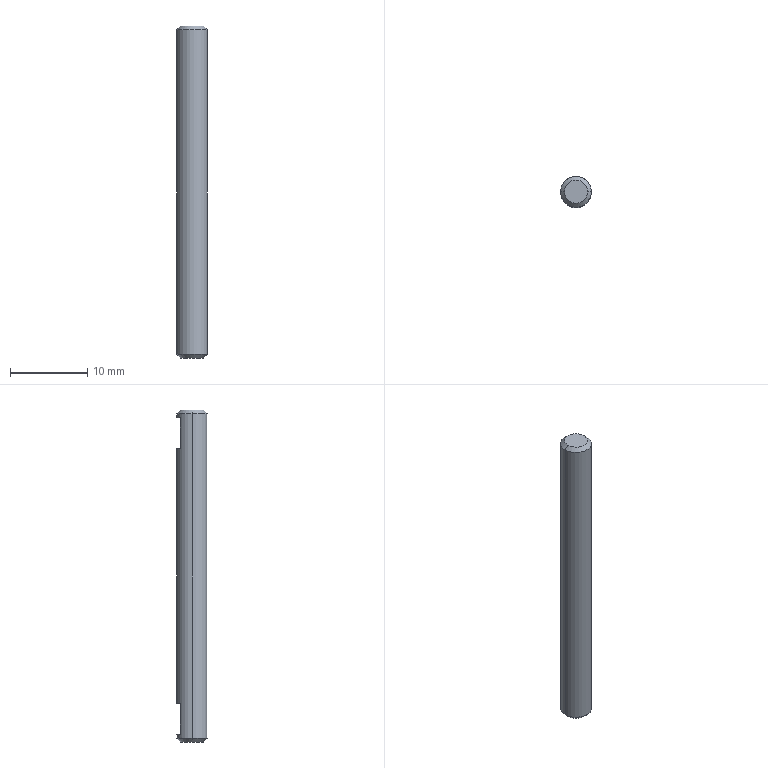Part | SolidWorks | features Chamfer 1, Extrusion 1, ICE 1 | 1 solid | 14 faces | box 4 x 4 x 43 mm | volume 530.221 mm3 | plane 8 | cone 4 | cylinder 2 | commonest cylinder face diameters 4 x2
STEP:
#1=CARTESIAN_POINT('',(-1.5,0.,-21.5));
#2=VERTEX_POINT('',#1);
#3=CARTESIAN_POINT('',(1.5,0.,-21.5));
#4=VERTEX_POINT('',#3);
#5=CARTESIAN_POINT('',(0.,0.,-21.5));
#6=DIRECTION('',(0.,0.,-1.));
#7=DIRECTION('',(1.,0.,0.));
#8=AXIS2_PLACEMENT_3D('',#5,#6,#7);
#9=CIRCLE('',#8,1.5);
#10=EDGE_CURVE('',#2,#4,#9,.T.);
#11=ORIENTED_EDGE('',*,*,#10,.F.);
#12=CARTESIAN_POINT('',(-2.,0.,-21.));
#13=VERTEX_POINT('',#12);
#14=CARTESIAN_POINT('',(-2.,0.,-21.));
#15=DIRECTION('',(-0.7071,0.,0.7071));
#16=VECTOR('',#15,1000.);
#17=LINE('',#14,#16);
#18=EDGE_CURVE('',#2,#13,#17,.T.);
#19=ORIENTED_EDGE('',*,*,#18,.T.);
#20=CARTESIAN_POINT('',(2.,0.,-21.));
#21=VERTEX_POINT('',#20);
#22=CARTESIAN_POINT('',(0.,0.,-21.));
#23=DIRECTION('',(0.,0.,1.));
#24=DIRECTION('',(1.,0.,0.));
#25=AXIS2_PLACEMENT_3D('',#22,#23,#24);
#26=CIRCLE('',#25,2.);
#27=EDGE_CURVE('',#21,#13,#26,.T.);
#28=ORIENTED_EDGE('',*,*,#27,.F.);
#29=CARTESIAN_POINT('',(2.,0.,-21.));
#30=DIRECTION('',(0.7071,0.,0.7071));
#31=VECTOR('',#30,1000.);
#32=LINE('',#29,#31);
#33=EDGE_CURVE('',#4,#21,#32,.T.);
#34=ORIENTED_EDGE('',*,*,#33,.F.);
#35=EDGE_LOOP('',(#11,#19,#28,#34));
#36=FACE_OUTER_BOUND('',#35,.T.);
#37=CARTESIAN_POINT('',(0.,0.,-21.));
#38=DIRECTION('',(0.,0.,1.));
#39=DIRECTION('',(1.,0.,0.));
#40=AXIS2_PLACEMENT_3D('',#37,#38,#39);
#41=CONICAL_SURFACE('',#40,2.,0.7854);
#42=ADVANCED_FACE('',(#36),#41,.T.);
#43=CARTESIAN_POINT('',(1.5,0.,21.5));
#44=VERTEX_POINT('',#43);
#45=CARTESIAN_POINT('',(-1.5,0.,21.5));
#46=VERTEX_POINT('',#45);
#47=CARTESIAN_POINT('',(0.,0.,21.5));
#48=DIRECTION('',(0.,0.,1.));
#49=DIRECTION('',(1.,0.,0.));
#50=AXIS2_PLACEMENT_3D('',#47,#48,#49);
#51=CIRCLE('',#50,1.5);
#52=EDGE_CURVE('',#44,#46,#51,.T.);
#53=ORIENTED_EDGE('',*,*,#52,.F.);
#54=CARTESIAN_POINT('',(2.,0.,21.));
#55=VERTEX_POINT('',#54);
#56=CARTESIAN_POINT('',(1.5,0.,21.5));
#57=DIRECTION('',(0.7071,0.,-0.7071));
#58=VECTOR('',#57,1000.);
#59=LINE('',#56,#58);
#60=EDGE_CURVE('',#44,#55,#59,.T.);
#61=ORIENTED_EDGE('',*,*,#60,.T.);
#62=CARTESIAN_POINT('',(-2.,0.,21.));
#63=VERTEX_POINT('',#62);
#64=CARTESIAN_POINT('',(0.,0.,21.));
#65=DIRECTION('',(0.,0.,-1.));
#66=DIRECTION('',(1.,0.,0.));
#67=AXIS2_PLACEMENT_3D('',#64,#65,#66);
#68=CIRCLE('',#67,2.);
#69=EDGE_CURVE('',#63,#55,#68,.T.);
#70=ORIENTED_EDGE('',*,*,#69,.F.);
#71=CARTESIAN_POINT('',(-1.5,0.,21.5));
#72=DIRECTION('',(-0.7071,0.,-0.7071));
#73=VECTOR('',#72,1000.);
#74=LINE('',#71,#73);
#75=EDGE_CURVE('',#46,#63,#74,.T.);
#76=ORIENTED_EDGE('',*,*,#75,.F.);
#77=EDGE_LOOP('',(#53,#61,#70,#76));
#78=FACE_OUTER_BOUND('',#77,.T.);
#79=CARTESIAN_POINT('',(0.,0.,21.5));
#80=DIRECTION('',(0.,0.,-1.));
#81=DIRECTION('',(-1.,0.,0.));
#82=AXIS2_PLACEMENT_3D('',#79,#80,#81);
#83=CONICAL_SURFACE('',#82,1.5,0.7854);
#84=ADVANCED_FACE('',(#78),#83,.T.);
#85=CARTESIAN_POINT('',(1.323,1.5,-16.5));
#86=VERTEX_POINT('',#85);
#87=CARTESIAN_POINT('',(1.323,1.5,-20.5));
#88=VERTEX_POINT('',#87);
#89=CARTESIAN_POINT('',(1.323,1.5,21.5));
#90=DIRECTION('',(0.,0.,-1.));
#91=VECTOR('',#90,1000.);
#92=LINE('',#89,#91);
#93=EDGE_CURVE('',#86,#88,#92,.T.);
#94=ORIENTED_EDGE('',*,*,#93,.F.);
#95=CARTESIAN_POINT('',(-1.323,1.5,-16.5));
#96=VERTEX_POINT('',#95);
#97=CARTESIAN_POINT('',(0.,0.,-16.5));
#98=DIRECTION('',(0.,0.,1.));
#99=DIRECTION('',(1.,0.,0.));
#100=AXIS2_PLACEMENT_3D('',#97,#98,#99);
#101=CIRCLE('',#100,2.);
#102=EDGE_CURVE('',#86,#96,#101,.T.);
#103=ORIENTED_EDGE('',*,*,#102,.T.);
#104=CARTESIAN_POINT('',(-1.323,1.5,-20.5));
#105=VERTEX_POINT('',#104);
#106=CARTESIAN_POINT('',(-1.323,1.5,21.5));
#107=DIRECTION('',(0.,0.,1.));
#108=VECTOR('',#107,1000.);
#109=LINE('',#106,#108);
#110=EDGE_CURVE('',#105,#96,#109,.T.);
#111=ORIENTED_EDGE('',*,*,#110,.F.);
#112=CARTESIAN_POINT('',(0.,0.,-20.5));
#113=DIRECTION('',(0.,0.,-1.));
#114=DIRECTION('',(-1.,0.,0.));
#115=AXIS2_PLACEMENT_3D('',#112,#113,#114);
#116=CIRCLE('',#115,2.);
#117=EDGE_CURVE('',#105,#88,#116,.T.);
#118=ORIENTED_EDGE('',*,*,#117,.T.);
#119=EDGE_LOOP('',(#94,#103,#111,#118));
#120=FACE_BOUND('',#119,.T.);
#121=CARTESIAN_POINT('',(1.323,1.5,20.5));
#122=VERTEX_POINT('',#121);
#123=CARTESIAN_POINT('',(1.323,1.5,16.5));
#124=VERTEX_POINT('',#123);
#125=CARTESIAN_POINT('',(1.323,1.5,21.5));
#126=DIRECTION('',(0.,0.,-1.));
#127=VECTOR('',#126,1000.);
#128=LINE('',#125,#127);
#129=EDGE_CURVE('',#122,#124,#128,.T.);
#130=ORIENTED_EDGE('',*,*,#129,.F.);
#131=CARTESIAN_POINT('',(-1.323,1.5,20.5));
#132=VERTEX_POINT('',#131);
#133=CARTESIAN_POINT('',(0.,0.,20.5));
#134=DIRECTION('',(0.,0.,1.));
#135=DIRECTION('',(1.,0.,0.));
#136=AXIS2_PLACEMENT_3D('',#133,#134,#135);
#137=CIRCLE('',#136,2.);
#138=EDGE_CURVE('',#122,#132,#137,.T.);
#139=ORIENTED_EDGE('',*,*,#138,.T.);
#140=CARTESIAN_POINT('',(-1.323,1.5,16.5));
#141=VERTEX_POINT('',#140);
#142=CARTESIAN_POINT('',(-1.323,1.5,21.5));
#143=DIRECTION('',(0.,0.,1.));
#144=VECTOR('',#143,1000.);
#145=LINE('',#142,#144);
#146=EDGE_CURVE('',#141,#132,#145,.T.);
#147=ORIENTED_EDGE('',*,*,#146,.F.);
#148=CARTESIAN_POINT('',(0.,0.,16.5));
#149=DIRECTION('',(0.,0.,-1.));
#150=DIRECTION('',(-1.,0.,0.));
#151=AXIS2_PLACEMENT_3D('',#148,#149,#150);
#152=CIRCLE('',#151,2.);
#153=EDGE_CURVE('',#141,#124,#152,.T.);
#154=ORIENTED_EDGE('',*,*,#153,.T.);
#155=EDGE_LOOP('',(#130,#139,#147,#154));
#156=FACE_BOUND('',#155,.T.);
#157=ORIENTED_EDGE('',*,*,#69,.T.);
#158=CARTESIAN_POINT('',(2.,0.,21.5));
#159=DIRECTION('',(0.,0.,-1.));
#160=VECTOR('',#159,1000.);
#161=LINE('',#158,#160);
#162=EDGE_CURVE('',#55,#21,#161,.T.);
#163=ORIENTED_EDGE('',*,*,#162,.T.);
#164=ORIENTED_EDGE('',*,*,#27,.T.);
#165=CARTESIAN_POINT('',(-2.,0.,21.5));
#166=DIRECTION('',(0.,0.,-1.));
#167=VECTOR('',#166,1000.);
#168=LINE('',#165,#167);
#169=EDGE_CURVE('',#63,#13,#168,.T.);
#170=ORIENTED_EDGE('',*,*,#169,.F.);
#171=EDGE_LOOP('',(#157,#163,#164,#170));
#172=FACE_OUTER_BOUND('',#171,.T.);
#173=CARTESIAN_POINT('',(0.,0.,21.5));
#174=DIRECTION('',(0.,0.,-1.));
#175=DIRECTION('',(-1.,0.,0.));
#176=AXIS2_PLACEMENT_3D('',#173,#174,#175);
#177=CYLINDRICAL_SURFACE('',#176,2.);
#178=ADVANCED_FACE('',(#120,#156,#172),#177,.T.);
#179=ORIENTED_EDGE('',*,*,#162,.F.);
#180=CARTESIAN_POINT('',(0.,0.,21.));
#181=DIRECTION('',(0.,0.,-1.));
#182=DIRECTION('',(1.,0.,0.));
#183=AXIS2_PLACEMENT_3D('',#180,#181,#182);
#184=CIRCLE('',#183,2.);
#185=EDGE_CURVE('',#55,#63,#184,.T.);
#186=ORIENTED_EDGE('',*,*,#185,.T.);
#187=ORIENTED_EDGE('',*,*,#169,.T.);
#188=CARTESIAN_POINT('',(0.,0.,-21.));
#189=DIRECTION('',(0.,0.,1.));
#190=DIRECTION('',(1.,0.,0.));
#191=AXIS2_PLACEMENT_3D('',#188,#189,#190);
#192=CIRCLE('',#191,2.);
#193=EDGE_CURVE('',#13,#21,#192,.T.);
#194=ORIENTED_EDGE('',*,*,#193,.T.);
#195=EDGE_LOOP('',(#179,#186,#187,#194));
#196=FACE_OUTER_BOUND('',#195,.T.);
#197=CARTESIAN_POINT('',(0.,0.,21.5));
#198=DIRECTION('',(0.,0.,-1.));
#199=DIRECTION('',(-1.,0.,0.));
#200=AXIS2_PLACEMENT_3D('',#197,#198,#199);
#201=CYLINDRICAL_SURFACE('',#200,2.);
#202=ADVANCED_FACE('',(#196),#201,.T.);
#203=CARTESIAN_POINT('',(0.,0.,21.5));
#204=DIRECTION('',(0.,0.,1.));
#205=DIRECTION('',(1.,0.,0.));
#206=AXIS2_PLACEMENT_3D('',#203,#204,#205);
#207=CIRCLE('',#206,1.5);
#208=EDGE_CURVE('',#46,#44,#207,.T.);
#209=ORIENTED_EDGE('',*,*,#208,.T.);
#210=ORIENTED_EDGE('',*,*,#52,.T.);
#211=EDGE_LOOP('',(#209,#210));
#212=FACE_OUTER_BOUND('',#211,.T.);
#213=CARTESIAN_POINT('',(0.,0.,21.5));
#214=DIRECTION('',(0.,0.,1.));
#215=DIRECTION('',(1.,0.,0.));
#216=AXIS2_PLACEMENT_3D('',#213,#214,#215);
#217=PLANE('',#216);
#218=ADVANCED_FACE('',(#212),#217,.T.);
#219=CARTESIAN_POINT('',(0.,0.,-21.5));
#220=DIRECTION('',(0.,0.,-1.));
#221=DIRECTION('',(1.,0.,0.));
#222=AXIS2_PLACEMENT_3D('',#219,#220,#221);
#223=CIRCLE('',#222,1.5);
#224=EDGE_CURVE('',#4,#2,#223,.T.);
#225=ORIENTED_EDGE('',*,*,#224,.T.);
#226=ORIENTED_EDGE('',*,*,#10,.T.);
#227=EDGE_LOOP('',(#225,#226));
#228=FACE_OUTER_BOUND('',#227,.T.);
#229=CARTESIAN_POINT('',(0.,0.,-21.5));
#230=DIRECTION('',(0.,0.,1.));
#231=DIRECTION('',(1.,0.,0.));
#232=AXIS2_PLACEMENT_3D('',#229,#230,#231);
#233=PLANE('',#232);
#234=ADVANCED_FACE('',(#228),#233,.F.);
#235=CARTESIAN_POINT('',(7.709,1.5,20.5));
#236=DIRECTION('',(1.,0.,0.));
#237=VECTOR('',#236,1000.);
#238=LINE('',#235,#237);
#239=EDGE_CURVE('',#132,#122,#238,.T.);
#240=ORIENTED_EDGE('',*,*,#239,.F.);
#241=ORIENTED_EDGE('',*,*,#138,.F.);
#242=EDGE_LOOP('',(#240,#241));
#243=FACE_OUTER_BOUND('',#242,.T.);
#244=CARTESIAN_POINT('',(7.709,1.5,20.5));
#245=DIRECTION('',(0.,0.,1.));
#246=DIRECTION('',(1.,0.,0.));
#247=AXIS2_PLACEMENT_3D('',#244,#245,#246);
#248=PLANE('',#247);
#249=ADVANCED_FACE('',(#243),#248,.F.);
#250=CARTESIAN_POINT('',(7.709,1.5,16.5));
#251=DIRECTION('',(-1.,0.,0.));
#252=VECTOR('',#251,1000.);
#253=LINE('',#250,#252);
#254=EDGE_CURVE('',#124,#141,#253,.T.);
#255=ORIENTED_EDGE('',*,*,#254,.F.);
#256=ORIENTED_EDGE('',*,*,#153,.F.);
#257=EDGE_LOOP('',(#255,#256));
#258=FACE_OUTER_BOUND('',#257,.T.);
#259=CARTESIAN_POINT('',(7.709,1.5,16.5));
#260=DIRECTION('',(0.,0.,-1.));
#261=DIRECTION('',(-1.,0.,0.));
#262=AXIS2_PLACEMENT_3D('',#259,#260,#261);
#263=PLANE('',#262);
#264=ADVANCED_FACE('',(#258),#263,.F.);
#265=ORIENTED_EDGE('',*,*,#129,.T.);
#266=ORIENTED_EDGE('',*,*,#254,.T.);
#267=ORIENTED_EDGE('',*,*,#146,.T.);
#268=ORIENTED_EDGE('',*,*,#239,.T.);
#269=EDGE_LOOP('',(#265,#266,#267,#268));
#270=FACE_OUTER_BOUND('',#269,.T.);
#271=CARTESIAN_POINT('',(7.709,1.5,16.5));
#272=DIRECTION('',(0.,1.,0.));
#273=DIRECTION('',(0.,0.,1.));
#274=AXIS2_PLACEMENT_3D('',#271,#272,#273);
#275=PLANE('',#274);
#276=ADVANCED_FACE('',(#270),#275,.T.);
#277=CARTESIAN_POINT('',(5.032,1.5,-16.5));
#278=DIRECTION('',(1.,0.,0.));
#279=VECTOR('',#278,1000.);
#280=LINE('',#277,#279);
#281=EDGE_CURVE('',#96,#86,#280,.T.);
#282=ORIENTED_EDGE('',*,*,#281,.F.);
#283=ORIENTED_EDGE('',*,*,#102,.F.);
#284=EDGE_LOOP('',(#282,#283));
#285=FACE_OUTER_BOUND('',#284,.T.);
#286=CARTESIAN_POINT('',(5.032,1.5,-16.5));
#287=DIRECTION('',(0.,0.,1.));
#288=DIRECTION('',(1.,0.,0.));
#289=AXIS2_PLACEMENT_3D('',#286,#287,#288);
#290=PLANE('',#289);
#291=ADVANCED_FACE('',(#285),#290,.F.);
#292=CARTESIAN_POINT('',(5.032,1.5,-20.5));
#293=DIRECTION('',(-1.,0.,0.));
#294=VECTOR('',#293,1000.);
#295=LINE('',#292,#294);
#296=EDGE_CURVE('',#88,#105,#295,.T.);
#297=ORIENTED_EDGE('',*,*,#296,.F.);
#298=ORIENTED_EDGE('',*,*,#117,.F.);
#299=EDGE_LOOP('',(#297,#298));
#300=FACE_OUTER_BOUND('',#299,.T.);
#301=CARTESIAN_POINT('',(5.032,1.5,-20.5));
#302=DIRECTION('',(0.,0.,-1.));
#303=DIRECTION('',(-1.,0.,0.));
#304=AXIS2_PLACEMENT_3D('',#301,#302,#303);
#305=PLANE('',#304);
#306=ADVANCED_FACE('',(#300),#305,.F.);
#307=ORIENTED_EDGE('',*,*,#93,.T.);
#308=ORIENTED_EDGE('',*,*,#296,.T.);
#309=ORIENTED_EDGE('',*,*,#110,.T.);
#310=ORIENTED_EDGE('',*,*,#281,.T.);
#311=EDGE_LOOP('',(#307,#308,#309,#310));
#312=FACE_OUTER_BOUND('',#311,.T.);
#313=CARTESIAN_POINT('',(5.032,1.5,-20.5));
#314=DIRECTION('',(0.,1.,0.));
#315=DIRECTION('',(0.,0.,1.));
#316=AXIS2_PLACEMENT_3D('',#313,#314,#315);
#317=PLANE('',#316);
#318=ADVANCED_FACE('',(#312),#317,.T.);
#319=ORIENTED_EDGE('',*,*,#60,.F.);
#320=ORIENTED_EDGE('',*,*,#208,.F.);
#321=ORIENTED_EDGE('',*,*,#75,.T.);
#322=ORIENTED_EDGE('',*,*,#185,.F.);
#323=EDGE_LOOP('',(#319,#320,#321,#322));
#324=FACE_OUTER_BOUND('',#323,.T.);
#325=CARTESIAN_POINT('',(0.,0.,21.5));
#326=DIRECTION('',(0.,0.,-1.));
#327=DIRECTION('',(-1.,0.,0.));
#328=AXIS2_PLACEMENT_3D('',#325,#326,#327);
#329=CONICAL_SURFACE('',#328,1.5,0.7854);
#330=ADVANCED_FACE('',(#324),#329,.T.);
#331=ORIENTED_EDGE('',*,*,#18,.F.);
#332=ORIENTED_EDGE('',*,*,#224,.F.);
#333=ORIENTED_EDGE('',*,*,#33,.T.);
#334=ORIENTED_EDGE('',*,*,#193,.F.);
#335=EDGE_LOOP('',(#331,#332,#333,#334));
#336=FACE_OUTER_BOUND('',#335,.T.);
#337=CARTESIAN_POINT('',(0.,0.,-21.));
#338=DIRECTION('',(0.,0.,1.));
#339=DIRECTION('',(1.,0.,0.));
#340=AXIS2_PLACEMENT_3D('',#337,#338,#339);
#341=CONICAL_SURFACE('',#340,2.,0.7854);
#342=ADVANCED_FACE('',(#336),#341,.T.);
#343=CLOSED_SHELL('',(#42,#84,#178,#202,#218,#234,#249,#264,#276,#291,#306,#318,#330,#342));
#344=MANIFOLD_SOLID_BREP('',#343);
#345=CARTESIAN_POINT('',(0.,0.,0.));
#346=DIRECTION('',(0.,0.,1.));
#347=DIRECTION('',(1.,0.,0.));
#348=AXIS2_PLACEMENT_3D('',#345,#346,#347);
#349=(LENGTH_UNIT()NAMED_UNIT(*)SI_UNIT(.MILLI.,.METRE.));
#350=UNCERTAINTY_MEASURE_WITH_UNIT(LENGTH_MEASURE(0.00001),#349,'','');
#351=(NAMED_UNIT(*)PLANE_ANGLE_UNIT()SI_UNIT($,.RADIAN.));
#352=(NAMED_UNIT(*)SI_UNIT($,.STERADIAN.)SOLID_ANGLE_UNIT());
#353=(GEOMETRIC_REPRESENTATION_CONTEXT(3)GLOBAL_UNCERTAINTY_ASSIGNED_CONTEXT((#350))GLOBAL_UNIT_ASSIGNED_CONTEXT((#349,#351,#352))REPRESENTATION_CONTEXT('',''));
#354=ADVANCED_BREP_SHAPE_REPRESENTATION('',(#344,#348),#353);